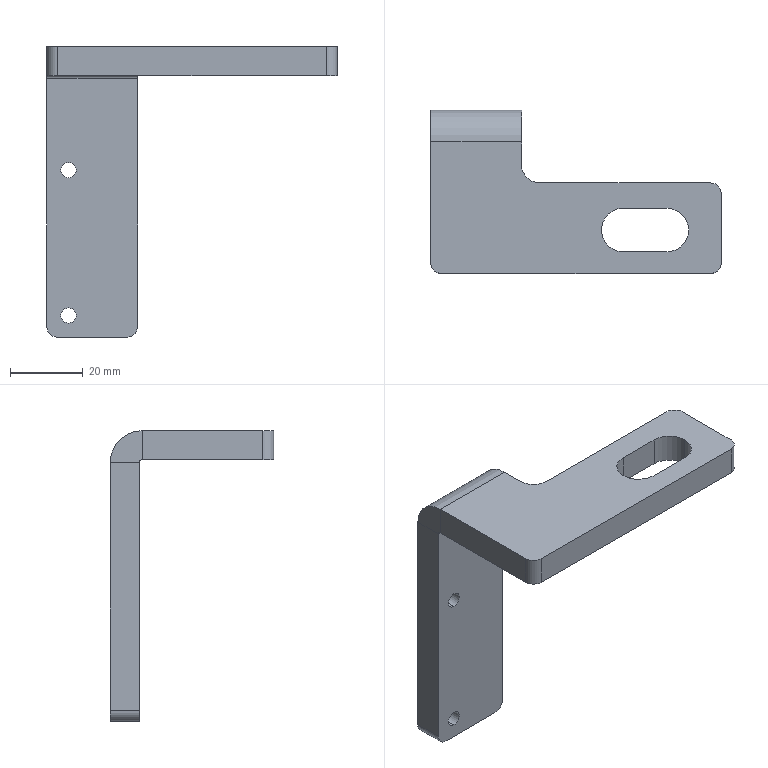Part | 1 solid | 31 faces | box 80 x 45 x 80 mm | volume 31681 mm3 | plane 16 | cylinder 15 | commonest cylinder face diameters 6 x5 4.2 x4 12 x3 1.473 x1 10 x1 17.473 x1
STEP:
#1=CARTESIAN_POINT('',(25.,-4.5,-8.));
#2=VERTEX_POINT('',#1);
#3=CARTESIAN_POINT('',(31.,-10.5,-8.));
#4=VERTEX_POINT('',#3);
#5=CARTESIAN_POINT('',(25.,-10.5,-8.));
#6=DIRECTION('',(0.,0.,-1.));
#7=DIRECTION('',(-1.,0.,0.));
#8=AXIS2_PLACEMENT_3D('',#5,#6,#7);
#9=CIRCLE('',#8,6.);
#10=EDGE_CURVE('',#2,#4,#9,.T.);
#11=ORIENTED_EDGE('',*,*,#10,.T.);
#12=CARTESIAN_POINT('',(31.,-10.5,0.));
#13=VERTEX_POINT('',#12);
#14=CARTESIAN_POINT('',(31.,-10.5,-30.));
#15=DIRECTION('',(0.,0.,1.));
#16=VECTOR('',#15,1000.);
#17=LINE('',#14,#16);
#18=EDGE_CURVE('',#4,#13,#17,.T.);
#19=ORIENTED_EDGE('',*,*,#18,.T.);
#20=CARTESIAN_POINT('',(25.,-4.5,0.));
#21=VERTEX_POINT('',#20);
#22=CARTESIAN_POINT('',(25.,-10.5,0.));
#23=DIRECTION('',(0.,0.,1.));
#24=DIRECTION('',(1.,0.,0.));
#25=AXIS2_PLACEMENT_3D('',#22,#23,#24);
#26=CIRCLE('',#25,6.);
#27=EDGE_CURVE('',#13,#21,#26,.T.);
#28=ORIENTED_EDGE('',*,*,#27,.T.);
#29=CARTESIAN_POINT('',(25.,-4.5,-30.));
#30=DIRECTION('',(0.,0.,1.));
#31=VECTOR('',#30,1000.);
#32=LINE('',#29,#31);
#33=EDGE_CURVE('',#2,#21,#32,.T.);
#34=ORIENTED_EDGE('',*,*,#33,.F.);
#35=EDGE_LOOP('',(#11,#19,#28,#34));
#36=FACE_OUTER_BOUND('',#35,.T.);
#37=CARTESIAN_POINT('',(25.,-10.5,-30.));
#38=DIRECTION('',(0.,0.,1.));
#39=DIRECTION('',(1.,0.,0.));
#40=AXIS2_PLACEMENT_3D('',#37,#38,#39);
#41=CYLINDRICAL_SURFACE('',#40,6.);
#42=ADVANCED_FACE('',(#36),#41,.F.);
#43=CARTESIAN_POINT('',(-34.,14.5,-76.1));
#44=VERTEX_POINT('',#43);
#45=CARTESIAN_POINT('',(-34.,14.5,-71.9));
#46=VERTEX_POINT('',#45);
#47=CARTESIAN_POINT('',(-34.,14.5,-74.));
#48=DIRECTION('',(0.,1.,0.));
#49=DIRECTION('',(0.,0.,1.));
#50=AXIS2_PLACEMENT_3D('',#47,#48,#49);
#51=CIRCLE('',#50,2.1);
#52=EDGE_CURVE('',#44,#46,#51,.T.);
#53=ORIENTED_EDGE('',*,*,#52,.F.);
#54=CARTESIAN_POINT('',(-34.,22.5,-76.1));
#55=VERTEX_POINT('',#54);
#56=CARTESIAN_POINT('',(-34.,22.5,-76.1));
#57=DIRECTION('',(0.,1.,0.));
#58=VECTOR('',#57,1000.);
#59=LINE('',#56,#58);
#60=EDGE_CURVE('',#44,#55,#59,.T.);
#61=ORIENTED_EDGE('',*,*,#60,.T.);
#62=CARTESIAN_POINT('',(-34.,22.5,-71.9));
#63=VERTEX_POINT('',#62);
#64=CARTESIAN_POINT('',(-34.,22.5,-74.));
#65=DIRECTION('',(0.,1.,0.));
#66=DIRECTION('',(0.,0.,1.));
#67=AXIS2_PLACEMENT_3D('',#64,#65,#66);
#68=CIRCLE('',#67,2.1);
#69=EDGE_CURVE('',#55,#63,#68,.T.);
#70=ORIENTED_EDGE('',*,*,#69,.T.);
#71=CARTESIAN_POINT('',(-34.,22.5,-71.9));
#72=DIRECTION('',(0.,1.,0.));
#73=VECTOR('',#72,1000.);
#74=LINE('',#71,#73);
#75=EDGE_CURVE('',#46,#63,#74,.T.);
#76=ORIENTED_EDGE('',*,*,#75,.F.);
#77=EDGE_LOOP('',(#53,#61,#70,#76));
#78=FACE_OUTER_BOUND('',#77,.T.);
#79=CARTESIAN_POINT('',(-34.,22.5,-74.));
#80=DIRECTION('',(0.,1.,0.));
#81=DIRECTION('',(0.,0.,1.));
#82=AXIS2_PLACEMENT_3D('',#79,#80,#81);
#83=CYLINDRICAL_SURFACE('',#82,2.1);
#84=ADVANCED_FACE('',(#78),#83,.F.);
#85=CARTESIAN_POINT('',(-34.,14.5,-36.1));
#86=VERTEX_POINT('',#85);
#87=CARTESIAN_POINT('',(-34.,14.5,-31.9));
#88=VERTEX_POINT('',#87);
#89=CARTESIAN_POINT('',(-34.,14.5,-34.));
#90=DIRECTION('',(0.,1.,0.));
#91=DIRECTION('',(0.,0.,1.));
#92=AXIS2_PLACEMENT_3D('',#89,#90,#91);
#93=CIRCLE('',#92,2.1);
#94=EDGE_CURVE('',#86,#88,#93,.T.);
#95=ORIENTED_EDGE('',*,*,#94,.F.);
#96=CARTESIAN_POINT('',(-34.,22.5,-36.1));
#97=VERTEX_POINT('',#96);
#98=CARTESIAN_POINT('',(-34.,22.5,-36.1));
#99=DIRECTION('',(0.,1.,0.));
#100=VECTOR('',#99,1000.);
#101=LINE('',#98,#100);
#102=EDGE_CURVE('',#86,#97,#101,.T.);
#103=ORIENTED_EDGE('',*,*,#102,.T.);
#104=CARTESIAN_POINT('',(-34.,22.5,-31.9));
#105=VERTEX_POINT('',#104);
#106=CARTESIAN_POINT('',(-34.,22.5,-34.));
#107=DIRECTION('',(0.,1.,0.));
#108=DIRECTION('',(0.,0.,1.));
#109=AXIS2_PLACEMENT_3D('',#106,#107,#108);
#110=CIRCLE('',#109,2.1);
#111=EDGE_CURVE('',#97,#105,#110,.T.);
#112=ORIENTED_EDGE('',*,*,#111,.T.);
#113=CARTESIAN_POINT('',(-34.,22.5,-31.9));
#114=DIRECTION('',(0.,1.,0.));
#115=VECTOR('',#114,1000.);
#116=LINE('',#113,#115);
#117=EDGE_CURVE('',#88,#105,#116,.T.);
#118=ORIENTED_EDGE('',*,*,#117,.F.);
#119=EDGE_LOOP('',(#95,#103,#112,#118));
#120=FACE_OUTER_BOUND('',#119,.T.);
#121=CARTESIAN_POINT('',(-34.,22.5,-34.));
#122=DIRECTION('',(0.,1.,0.));
#123=DIRECTION('',(0.,0.,1.));
#124=AXIS2_PLACEMENT_3D('',#121,#122,#123);
#125=CYLINDRICAL_SURFACE('',#124,2.1);
#126=ADVANCED_FACE('',(#120),#125,.F.);
#127=CARTESIAN_POINT('',(-15.,7.5,0.));
#128=VERTEX_POINT('',#127);
#129=CARTESIAN_POINT('',(-15.,13.763,0.));
#130=VERTEX_POINT('',#129);
#131=CARTESIAN_POINT('',(-15.,2.5,0.));
#132=DIRECTION('',(0.,1.,0.));
#133=VECTOR('',#132,1000.);
#134=LINE('',#131,#133);
#135=EDGE_CURVE('',#128,#130,#134,.T.);
#136=ORIENTED_EDGE('',*,*,#135,.F.);
#137=CARTESIAN_POINT('',(-15.,7.5,-8.));
#138=VERTEX_POINT('',#137);
#139=CARTESIAN_POINT('',(-15.,7.5,-8.));
#140=DIRECTION('',(0.,0.,-1.));
#141=VECTOR('',#140,1000.);
#142=LINE('',#139,#141);
#143=EDGE_CURVE('',#128,#138,#142,.T.);
#144=ORIENTED_EDGE('',*,*,#143,.T.);
#145=CARTESIAN_POINT('',(-15.,13.763,-8.));
#146=VERTEX_POINT('',#145);
#147=CARTESIAN_POINT('',(-15.,0.,-8.));
#148=DIRECTION('',(0.,1.,0.));
#149=VECTOR('',#148,1000.);
#150=LINE('',#147,#149);
#151=EDGE_CURVE('',#138,#146,#150,.T.);
#152=ORIENTED_EDGE('',*,*,#151,.T.);
#153=CARTESIAN_POINT('',(-15.,13.763,-8.));
#154=DIRECTION('',(0.,0.,1.));
#155=VECTOR('',#154,1000.);
#156=LINE('',#153,#155);
#157=EDGE_CURVE('',#146,#130,#156,.T.);
#158=ORIENTED_EDGE('',*,*,#157,.T.);
#159=EDGE_LOOP('',(#136,#144,#152,#158));
#160=FACE_OUTER_BOUND('',#159,.T.);
#161=CARTESIAN_POINT('',(-15.,2.5,0.));
#162=DIRECTION('',(-1.,0.,0.));
#163=DIRECTION('',(0.,0.,1.));
#164=AXIS2_PLACEMENT_3D('',#161,#162,#163);
#165=PLANE('',#164);
#166=ADVANCED_FACE('',(#160),#165,.F.);
#167=CARTESIAN_POINT('',(-15.,14.5,-77.));
#168=VERTEX_POINT('',#167);
#169=CARTESIAN_POINT('',(-15.,14.5,-8.737));
#170=VERTEX_POINT('',#169);
#171=CARTESIAN_POINT('',(-15.,14.5,0.));
#172=DIRECTION('',(0.,0.,1.));
#173=VECTOR('',#172,1000.);
#174=LINE('',#171,#173);
#175=EDGE_CURVE('',#168,#170,#174,.T.);
#176=ORIENTED_EDGE('',*,*,#175,.F.);
#177=CARTESIAN_POINT('',(-15.,22.5,-77.));
#178=VERTEX_POINT('',#177);
#179=CARTESIAN_POINT('',(-15.,22.5,-77.));
#180=DIRECTION('',(0.,1.,0.));
#181=VECTOR('',#180,1000.);
#182=LINE('',#179,#181);
#183=EDGE_CURVE('',#168,#178,#182,.T.);
#184=ORIENTED_EDGE('',*,*,#183,.T.);
#185=CARTESIAN_POINT('',(-15.,22.5,-8.737));
#186=VERTEX_POINT('',#185);
#187=CARTESIAN_POINT('',(-15.,22.5,0.));
#188=DIRECTION('',(0.,0.,1.));
#189=VECTOR('',#188,1000.);
#190=LINE('',#187,#189);
#191=EDGE_CURVE('',#178,#186,#190,.T.);
#192=ORIENTED_EDGE('',*,*,#191,.T.);
#193=CARTESIAN_POINT('',(-15.,22.5,-8.737));
#194=DIRECTION('',(0.,-1.,0.));
#195=VECTOR('',#194,1000.);
#196=LINE('',#193,#195);
#197=EDGE_CURVE('',#186,#170,#196,.T.);
#198=ORIENTED_EDGE('',*,*,#197,.T.);
#199=EDGE_LOOP('',(#176,#184,#192,#198));
#200=FACE_OUTER_BOUND('',#199,.T.);
#201=CARTESIAN_POINT('',(-15.,2.5,0.));
#202=DIRECTION('',(-1.,0.,0.));
#203=DIRECTION('',(0.,0.,1.));
#204=AXIS2_PLACEMENT_3D('',#201,#202,#203);
#205=PLANE('',#204);
#206=ADVANCED_FACE('',(#200),#205,.F.);
#207=CARTESIAN_POINT('',(40.,-19.5,0.));
#208=VERTEX_POINT('',#207);
#209=CARTESIAN_POINT('',(40.,-0.5,0.));
#210=VERTEX_POINT('',#209);
#211=CARTESIAN_POINT('',(40.,-22.5,0.));
#212=DIRECTION('',(0.,1.,0.));
#213=VECTOR('',#212,1000.);
#214=LINE('',#211,#213);
#215=EDGE_CURVE('',#208,#210,#214,.T.);
#216=ORIENTED_EDGE('',*,*,#215,.F.);
#217=CARTESIAN_POINT('',(40.,-19.5,-8.));
#218=VERTEX_POINT('',#217);
#219=CARTESIAN_POINT('',(40.,-19.5,-8.));
#220=DIRECTION('',(0.,0.,-1.));
#221=VECTOR('',#220,1000.);
#222=LINE('',#219,#221);
#223=EDGE_CURVE('',#208,#218,#222,.T.);
#224=ORIENTED_EDGE('',*,*,#223,.T.);
#225=CARTESIAN_POINT('',(40.,-0.5,-8.));
#226=VERTEX_POINT('',#225);
#227=CARTESIAN_POINT('',(40.,-22.5,-8.));
#228=DIRECTION('',(0.,1.,0.));
#229=VECTOR('',#228,1000.);
#230=LINE('',#227,#229);
#231=EDGE_CURVE('',#218,#226,#230,.T.);
#232=ORIENTED_EDGE('',*,*,#231,.T.);
#233=CARTESIAN_POINT('',(40.,-0.5,0.));
#234=DIRECTION('',(0.,0.,1.));
#235=VECTOR('',#234,1000.);
#236=LINE('',#233,#235);
#237=EDGE_CURVE('',#226,#210,#236,.T.);
#238=ORIENTED_EDGE('',*,*,#237,.T.);
#239=EDGE_LOOP('',(#216,#224,#232,#238));
#240=FACE_OUTER_BOUND('',#239,.T.);
#241=CARTESIAN_POINT('',(40.,-22.5,-8.));
#242=DIRECTION('',(1.,0.,0.));
#243=DIRECTION('',(0.,0.,-1.));
#244=AXIS2_PLACEMENT_3D('',#241,#242,#243);
#245=PLANE('',#244);
#246=ADVANCED_FACE('',(#240),#245,.T.);
#247=ORIENTED_EDGE('',*,*,#10,.F.);
#248=CARTESIAN_POINT('',(13.,-4.5,-8.));
#249=VERTEX_POINT('',#248);
#250=CARTESIAN_POINT('',(0.,-4.5,-8.));
#251=DIRECTION('',(1.,0.,0.));
#252=VECTOR('',#251,1000.);
#253=LINE('',#250,#252);
#254=EDGE_CURVE('',#249,#2,#253,.T.);
#255=ORIENTED_EDGE('',*,*,#254,.F.);
#256=CARTESIAN_POINT('',(13.,-16.5,-8.));
#257=VERTEX_POINT('',#256);
#258=CARTESIAN_POINT('',(13.,-10.5,-8.));
#259=DIRECTION('',(0.,0.,-1.));
#260=DIRECTION('',(-1.,0.,0.));
#261=AXIS2_PLACEMENT_3D('',#258,#259,#260);
#262=CIRCLE('',#261,6.);
#263=EDGE_CURVE('',#257,#249,#262,.T.);
#264=ORIENTED_EDGE('',*,*,#263,.F.);
#265=CARTESIAN_POINT('',(25.,-16.5,-8.));
#266=VERTEX_POINT('',#265);
#267=CARTESIAN_POINT('',(0.,-16.5,-8.));
#268=DIRECTION('',(-1.,0.,0.));
#269=VECTOR('',#268,1000.);
#270=LINE('',#267,#269);
#271=EDGE_CURVE('',#266,#257,#270,.T.);
#272=ORIENTED_EDGE('',*,*,#271,.F.);
#273=CARTESIAN_POINT('',(25.,-10.5,-8.));
#274=DIRECTION('',(0.,0.,-1.));
#275=DIRECTION('',(-1.,0.,0.));
#276=AXIS2_PLACEMENT_3D('',#273,#274,#275);
#277=CIRCLE('',#276,6.);
#278=EDGE_CURVE('',#4,#266,#277,.T.);
#279=ORIENTED_EDGE('',*,*,#278,.F.);
#280=EDGE_LOOP('',(#247,#255,#264,#272,#279));
#281=FACE_BOUND('',#280,.T.);
#282=CARTESIAN_POINT('',(-37.,-22.5,-8.));
#283=VERTEX_POINT('',#282);
#284=CARTESIAN_POINT('',(37.,-22.5,-8.));
#285=VERTEX_POINT('',#284);
#286=CARTESIAN_POINT('',(-40.,-22.5,-8.));
#287=DIRECTION('',(1.,0.,0.));
#288=VECTOR('',#287,1000.);
#289=LINE('',#286,#288);
#290=EDGE_CURVE('',#283,#285,#289,.T.);
#291=ORIENTED_EDGE('',*,*,#290,.F.);
#292=CARTESIAN_POINT('',(-40.,-19.5,-8.));
#293=VERTEX_POINT('',#292);
#294=CARTESIAN_POINT('',(-37.,-19.5,-8.));
#295=DIRECTION('',(0.,0.,-1.));
#296=DIRECTION('',(-1.,0.,0.));
#297=AXIS2_PLACEMENT_3D('',#294,#295,#296);
#298=CIRCLE('',#297,3.);
#299=EDGE_CURVE('',#283,#293,#298,.T.);
#300=ORIENTED_EDGE('',*,*,#299,.T.);
#301=CARTESIAN_POINT('',(-40.,13.763,-8.));
#302=VERTEX_POINT('',#301);
#303=CARTESIAN_POINT('',(-40.,-22.5,-8.));
#304=DIRECTION('',(0.,-1.,0.));
#305=VECTOR('',#304,1000.);
#306=LINE('',#303,#305);
#307=EDGE_CURVE('',#302,#293,#306,.T.);
#308=ORIENTED_EDGE('',*,*,#307,.F.);
#309=CARTESIAN_POINT('',(40.,13.763,-8.));
#310=DIRECTION('',(-1.,0.,0.));
#311=VECTOR('',#310,1000.);
#312=LINE('',#309,#311);
#313=EDGE_CURVE('',#146,#302,#312,.T.);
#314=ORIENTED_EDGE('',*,*,#313,.F.);
#315=ORIENTED_EDGE('',*,*,#151,.F.);
#316=CARTESIAN_POINT('',(-10.,2.5,-8.));
#317=VERTEX_POINT('',#316);
#318=CARTESIAN_POINT('',(-10.,7.5,-8.));
#319=DIRECTION('',(0.,0.,1.));
#320=DIRECTION('',(-1.,0.,0.));
#321=AXIS2_PLACEMENT_3D('',#318,#319,#320);
#322=CIRCLE('',#321,5.);
#323=EDGE_CURVE('',#138,#317,#322,.T.);
#324=ORIENTED_EDGE('',*,*,#323,.T.);
#325=CARTESIAN_POINT('',(37.,2.5,-8.));
#326=VERTEX_POINT('',#325);
#327=CARTESIAN_POINT('',(0.,2.5,-8.));
#328=DIRECTION('',(-1.,0.,0.));
#329=VECTOR('',#328,1000.);
#330=LINE('',#327,#329);
#331=EDGE_CURVE('',#326,#317,#330,.T.);
#332=ORIENTED_EDGE('',*,*,#331,.F.);
#333=CARTESIAN_POINT('',(37.,-0.5,-8.));
#334=DIRECTION('',(0.,0.,-1.));
#335=DIRECTION('',(-1.,0.,0.));
#336=AXIS2_PLACEMENT_3D('',#333,#334,#335);
#337=CIRCLE('',#336,3.);
#338=EDGE_CURVE('',#326,#226,#337,.T.);
#339=ORIENTED_EDGE('',*,*,#338,.T.);
#340=ORIENTED_EDGE('',*,*,#231,.F.);
#341=CARTESIAN_POINT('',(37.,-19.5,-8.));
#342=DIRECTION('',(0.,0.,-1.));
#343=DIRECTION('',(-1.,0.,0.));
#344=AXIS2_PLACEMENT_3D('',#341,#342,#343);
#345=CIRCLE('',#344,3.);
#346=EDGE_CURVE('',#218,#285,#345,.T.);
#347=ORIENTED_EDGE('',*,*,#346,.T.);
#348=EDGE_LOOP('',(#291,#300,#308,#314,#315,#324,#332,#339,#340,#347));
#349=FACE_OUTER_BOUND('',#348,.T.);
#350=CARTESIAN_POINT('',(0.,0.,-8.));
#351=DIRECTION('',(0.,0.,-1.));
#352=DIRECTION('',(-1.,0.,0.));
#353=AXIS2_PLACEMENT_3D('',#350,#351,#352);
#354=PLANE('',#353);
#355=ADVANCED_FACE('',(#281,#349),#354,.T.);
#356=CARTESIAN_POINT('',(13.,-4.5,0.));
#357=VERTEX_POINT('',#356);
#358=CARTESIAN_POINT('',(25.,-4.5,0.));
#359=DIRECTION('',(-1.,0.,0.));
#360=VECTOR('',#359,1000.);
#361=LINE('',#358,#360);
#362=EDGE_CURVE('',#21,#357,#361,.T.);
#363=ORIENTED_EDGE('',*,*,#362,.F.);
#364=ORIENTED_EDGE('',*,*,#27,.F.);
#365=CARTESIAN_POINT('',(25.,-16.5,0.));
#366=VERTEX_POINT('',#365);
#367=CARTESIAN_POINT('',(25.,-10.5,0.));
#368=DIRECTION('',(0.,0.,1.));
#369=DIRECTION('',(1.,0.,0.));
#370=AXIS2_PLACEMENT_3D('',#367,#368,#369);
#371=CIRCLE('',#370,6.);
#372=EDGE_CURVE('',#366,#13,#371,.T.);
#373=ORIENTED_EDGE('',*,*,#372,.F.);
#374=CARTESIAN_POINT('',(13.,-16.5,0.));
#375=VERTEX_POINT('',#374);
#376=CARTESIAN_POINT('',(25.,-16.5,0.));
#377=DIRECTION('',(1.,0.,0.));
#378=VECTOR('',#377,1000.);
#379=LINE('',#376,#378);
#380=EDGE_CURVE('',#375,#366,#379,.T.);
#381=ORIENTED_EDGE('',*,*,#380,.F.);
#382=CARTESIAN_POINT('',(13.,-10.5,0.));
#383=DIRECTION('',(0.,0.,1.));
#384=DIRECTION('',(1.,0.,0.));
#385=AXIS2_PLACEMENT_3D('',#382,#383,#384);
#386=CIRCLE('',#385,6.);
#387=EDGE_CURVE('',#357,#375,#386,.T.);
#388=ORIENTED_EDGE('',*,*,#387,.F.);
#389=EDGE_LOOP('',(#363,#364,#373,#381,#388));
#390=FACE_BOUND('',#389,.T.);
#391=CARTESIAN_POINT('',(-40.,13.763,0.));
#392=VERTEX_POINT('',#391);
#393=CARTESIAN_POINT('',(-40.,-19.5,0.));
#394=VERTEX_POINT('',#393);
#395=CARTESIAN_POINT('',(-40.,-22.5,0.));
#396=DIRECTION('',(0.,-1.,0.));
#397=VECTOR('',#396,1000.);
#398=LINE('',#395,#397);
#399=EDGE_CURVE('',#392,#394,#398,.T.);
#400=ORIENTED_EDGE('',*,*,#399,.T.);
#401=CARTESIAN_POINT('',(-37.,-22.5,0.));
#402=VERTEX_POINT('',#401);
#403=CARTESIAN_POINT('',(-37.,-19.5,0.));
#404=DIRECTION('',(0.,0.,1.));
#405=DIRECTION('',(-1.,0.,0.));
#406=AXIS2_PLACEMENT_3D('',#403,#404,#405);
#407=CIRCLE('',#406,3.);
#408=EDGE_CURVE('',#394,#402,#407,.T.);
#409=ORIENTED_EDGE('',*,*,#408,.T.);
#410=CARTESIAN_POINT('',(37.,-22.5,0.));
#411=VERTEX_POINT('',#410);
#412=CARTESIAN_POINT('',(-40.,-22.5,0.));
#413=DIRECTION('',(1.,0.,0.));
#414=VECTOR('',#413,1000.);
#415=LINE('',#412,#414);
#416=EDGE_CURVE('',#402,#411,#415,.T.);
#417=ORIENTED_EDGE('',*,*,#416,.T.);
#418=CARTESIAN_POINT('',(37.,-19.5,0.));
#419=DIRECTION('',(0.,0.,1.));
#420=DIRECTION('',(-1.,0.,0.));
#421=AXIS2_PLACEMENT_3D('',#418,#419,#420);
#422=CIRCLE('',#421,3.);
#423=EDGE_CURVE('',#411,#208,#422,.T.);
#424=ORIENTED_EDGE('',*,*,#423,.T.);
#425=ORIENTED_EDGE('',*,*,#215,.T.);
#426=CARTESIAN_POINT('',(37.,2.5,0.));
#427=VERTEX_POINT('',#426);
#428=CARTESIAN_POINT('',(37.,-0.5,0.));
#429=DIRECTION('',(0.,0.,1.));
#430=DIRECTION('',(-1.,0.,0.));
#431=AXIS2_PLACEMENT_3D('',#428,#429,#430);
#432=CIRCLE('',#431,3.);
#433=EDGE_CURVE('',#210,#427,#432,.T.);
#434=ORIENTED_EDGE('',*,*,#433,.T.);
#435=CARTESIAN_POINT('',(-10.,2.5,0.));
#436=VERTEX_POINT('',#435);
#437=CARTESIAN_POINT('',(-15.,2.5,0.));
#438=DIRECTION('',(1.,0.,0.));
#439=VECTOR('',#438,1000.);
#440=LINE('',#437,#439);
#441=EDGE_CURVE('',#436,#427,#440,.T.);
#442=ORIENTED_EDGE('',*,*,#441,.F.);
#443=CARTESIAN_POINT('',(-10.,7.5,0.));
#444=DIRECTION('',(0.,0.,-1.));
#445=DIRECTION('',(-1.,0.,0.));
#446=AXIS2_PLACEMENT_3D('',#443,#444,#445);
#447=CIRCLE('',#446,5.);
#448=EDGE_CURVE('',#436,#128,#447,.T.);
#449=ORIENTED_EDGE('',*,*,#448,.T.);
#450=ORIENTED_EDGE('',*,*,#135,.T.);
#451=CARTESIAN_POINT('',(40.,13.763,0.));
#452=DIRECTION('',(-1.,0.,0.));
#453=VECTOR('',#452,1000.);
#454=LINE('',#451,#453);
#455=EDGE_CURVE('',#130,#392,#454,.T.);
#456=ORIENTED_EDGE('',*,*,#455,.T.);
#457=EDGE_LOOP('',(#400,#409,#417,#424,#425,#434,#442,#449,#450,#456));
#458=FACE_OUTER_BOUND('',#457,.T.);
#459=CARTESIAN_POINT('',(0.,0.,0.));
#460=DIRECTION('',(0.,0.,-1.));
#461=DIRECTION('',(-1.,0.,0.));
#462=AXIS2_PLACEMENT_3D('',#459,#460,#461);
#463=PLANE('',#462);
#464=ADVANCED_FACE('',(#390,#458),#463,.F.);
#465=ORIENTED_EDGE('',*,*,#416,.F.);
#466=CARTESIAN_POINT('',(-37.,-22.5,-8.));
#467=DIRECTION('',(0.,0.,-1.));
#468=VECTOR('',#467,1000.);
#469=LINE('',#466,#468);
#470=EDGE_CURVE('',#402,#283,#469,.T.);
#471=ORIENTED_EDGE('',*,*,#470,.T.);
#472=ORIENTED_EDGE('',*,*,#290,.T.);
#473=CARTESIAN_POINT('',(37.,-22.5,-8.));
#474=DIRECTION('',(0.,0.,1.));
#475=VECTOR('',#474,1000.);
#476=LINE('',#473,#475);
#477=EDGE_CURVE('',#285,#411,#476,.T.);
#478=ORIENTED_EDGE('',*,*,#477,.T.);
#479=EDGE_LOOP('',(#465,#471,#472,#478));
#480=FACE_OUTER_BOUND('',#479,.T.);
#481=CARTESIAN_POINT('',(-40.,-22.5,-8.));
#482=DIRECTION('',(0.,-1.,0.));
#483=DIRECTION('',(0.,0.,-1.));
#484=AXIS2_PLACEMENT_3D('',#481,#482,#483);
#485=PLANE('',#484);
#486=ADVANCED_FACE('',(#480),#485,.T.);
#487=ORIENTED_EDGE('',*,*,#307,.T.);
#488=CARTESIAN_POINT('',(-40.,-19.5,-8.));
#489=DIRECTION('',(0.,0.,1.));
#490=VECTOR('',#489,1000.);
#491=LINE('',#488,#490);
#492=EDGE_CURVE('',#293,#394,#491,.T.);
#493=ORIENTED_EDGE('',*,*,#492,.T.);
#494=ORIENTED_EDGE('',*,*,#399,.F.);
#495=CARTESIAN_POINT('',(-40.,13.763,-8.));
#496=DIRECTION('',(0.,0.,1.));
#497=VECTOR('',#496,1000.);
#498=LINE('',#495,#497);
#499=EDGE_CURVE('',#302,#392,#498,.T.);
#500=ORIENTED_EDGE('',*,*,#499,.F.);
#501=EDGE_LOOP('',(#487,#493,#494,#500));
#502=FACE_OUTER_BOUND('',#501,.T.);
#503=CARTESIAN_POINT('',(-40.,-22.5,-8.));
#504=DIRECTION('',(-1.,0.,0.));
#505=DIRECTION('',(0.,0.,1.));
#506=AXIS2_PLACEMENT_3D('',#503,#504,#505);
#507=PLANE('',#506);
#508=ADVANCED_FACE('',(#502),#507,.T.);
#509=CARTESIAN_POINT('',(-40.,14.5,-8.737));
#510=VERTEX_POINT('',#509);
#511=CARTESIAN_POINT('',(-40.,22.5,-8.737));
#512=VERTEX_POINT('',#511);
#513=CARTESIAN_POINT('',(-40.,22.5,-8.737));
#514=DIRECTION('',(0.,1.,0.));
#515=VECTOR('',#514,1000.);
#516=LINE('',#513,#515);
#517=EDGE_CURVE('',#510,#512,#516,.T.);
#518=ORIENTED_EDGE('',*,*,#517,.F.);
#519=CARTESIAN_POINT('',(-40.,13.763,-8.737));
#520=DIRECTION('',(-1.,0.,0.));
#521=DIRECTION('',(0.,0.,-1.));
#522=AXIS2_PLACEMENT_3D('',#519,#520,#521);
#523=CIRCLE('',#522,0.7366);
#524=EDGE_CURVE('',#302,#510,#523,.T.);
#525=ORIENTED_EDGE('',*,*,#524,.F.);
#526=ORIENTED_EDGE('',*,*,#499,.T.);
#527=CARTESIAN_POINT('',(-40.,13.763,-8.737));
#528=DIRECTION('',(-1.,0.,0.));
#529=DIRECTION('',(0.,0.,-1.));
#530=AXIS2_PLACEMENT_3D('',#527,#528,#529);
#531=CIRCLE('',#530,8.737);
#532=EDGE_CURVE('',#392,#512,#531,.T.);
#533=ORIENTED_EDGE('',*,*,#532,.T.);
#534=EDGE_LOOP('',(#518,#525,#526,#533));
#535=FACE_OUTER_BOUND('',#534,.T.);
#536=CARTESIAN_POINT('',(-40.,13.763,-8.737));
#537=DIRECTION('',(-1.,0.,0.));
#538=DIRECTION('',(0.,0.,1.));
#539=AXIS2_PLACEMENT_3D('',#536,#537,#538);
#540=PLANE('',#539);
#541=ADVANCED_FACE('',(#535),#540,.T.);
#542=CARTESIAN_POINT('',(-15.,13.763,-8.737));
#543=DIRECTION('',(1.,0.,0.));
#544=DIRECTION('',(0.,0.,1.));
#545=AXIS2_PLACEMENT_3D('',#542,#543,#544);
#546=CIRCLE('',#545,8.737);
#547=EDGE_CURVE('',#186,#130,#546,.T.);
#548=ORIENTED_EDGE('',*,*,#547,.F.);
#549=CARTESIAN_POINT('',(0.,22.5,-8.737));
#550=DIRECTION('',(1.,0.,0.));
#551=VECTOR('',#550,1000.);
#552=LINE('',#549,#551);
#553=EDGE_CURVE('',#512,#186,#552,.T.);
#554=ORIENTED_EDGE('',*,*,#553,.F.);
#555=ORIENTED_EDGE('',*,*,#532,.F.);
#556=ORIENTED_EDGE('',*,*,#455,.F.);
#557=EDGE_LOOP('',(#548,#554,#555,#556));
#558=FACE_OUTER_BOUND('',#557,.T.);
#559=CARTESIAN_POINT('',(40.,13.763,-8.737));
#560=DIRECTION('',(1.,0.,0.));
#561=DIRECTION('',(0.,1.,0.));
#562=AXIS2_PLACEMENT_3D('',#559,#560,#561);
#563=CYLINDRICAL_SURFACE('',#562,8.737);
#564=ADVANCED_FACE('',(#558),#563,.T.);
#565=CARTESIAN_POINT('',(-40.,14.5,-8.737));
#566=DIRECTION('',(1.,0.,0.));
#567=VECTOR('',#566,1000.);
#568=LINE('',#565,#567);
#569=EDGE_CURVE('',#510,#170,#568,.T.);
#570=ORIENTED_EDGE('',*,*,#569,.T.);
#571=CARTESIAN_POINT('',(-15.,13.763,-8.737));
#572=DIRECTION('',(1.,0.,0.));
#573=DIRECTION('',(0.,0.,1.));
#574=AXIS2_PLACEMENT_3D('',#571,#572,#573);
#575=CIRCLE('',#574,0.7366);
#576=EDGE_CURVE('',#170,#146,#575,.T.);
#577=ORIENTED_EDGE('',*,*,#576,.T.);
#578=ORIENTED_EDGE('',*,*,#313,.T.);
#579=ORIENTED_EDGE('',*,*,#524,.T.);
#580=EDGE_LOOP('',(#570,#577,#578,#579));
#581=FACE_OUTER_BOUND('',#580,.T.);
#582=CARTESIAN_POINT('',(40.,13.763,-8.737));
#583=DIRECTION('',(1.,0.,0.));
#584=DIRECTION('',(0.,1.,0.));
#585=AXIS2_PLACEMENT_3D('',#582,#583,#584);
#586=CYLINDRICAL_SURFACE('',#585,0.7366);
#587=ADVANCED_FACE('',(#581),#586,.F.);
#588=CARTESIAN_POINT('',(-40.,22.5,-77.));
#589=VERTEX_POINT('',#588);
#590=CARTESIAN_POINT('',(-40.,22.5,-80.));
#591=DIRECTION('',(0.,0.,-1.));
#592=VECTOR('',#591,1000.);
#593=LINE('',#590,#592);
#594=EDGE_CURVE('',#512,#589,#593,.T.);
#595=ORIENTED_EDGE('',*,*,#594,.T.);
#596=CARTESIAN_POINT('',(-40.,14.5,-77.));
#597=VERTEX_POINT('',#596);
#598=CARTESIAN_POINT('',(-40.,22.5,-77.));
#599=DIRECTION('',(0.,-1.,0.));
#600=VECTOR('',#599,1000.);
#601=LINE('',#598,#600);
#602=EDGE_CURVE('',#589,#597,#601,.T.);
#603=ORIENTED_EDGE('',*,*,#602,.T.);
#604=CARTESIAN_POINT('',(-40.,14.5,0.));
#605=DIRECTION('',(0.,0.,-1.));
#606=VECTOR('',#605,1000.);
#607=LINE('',#604,#606);
#608=EDGE_CURVE('',#510,#597,#607,.T.);
#609=ORIENTED_EDGE('',*,*,#608,.F.);
#610=ORIENTED_EDGE('',*,*,#517,.T.);
#611=EDGE_LOOP('',(#595,#603,#609,#610));
#612=FACE_OUTER_BOUND('',#611,.T.);
#613=CARTESIAN_POINT('',(-40.,22.5,-80.));
#614=DIRECTION('',(-1.,0.,0.));
#615=DIRECTION('',(0.,0.,1.));
#616=AXIS2_PLACEMENT_3D('',#613,#614,#615);
#617=PLANE('',#616);
#618=ADVANCED_FACE('',(#612),#617,.T.);
#619=CARTESIAN_POINT('',(-37.,22.5,-80.));
#620=VERTEX_POINT('',#619);
#621=CARTESIAN_POINT('',(-18.,22.5,-80.));
#622=VERTEX_POINT('',#621);
#623=CARTESIAN_POINT('',(40.,22.5,-80.));
#624=DIRECTION('',(1.,0.,0.));
#625=VECTOR('',#624,1000.);
#626=LINE('',#623,#625);
#627=EDGE_CURVE('',#620,#622,#626,.T.);
#628=ORIENTED_EDGE('',*,*,#627,.F.);
#629=CARTESIAN_POINT('',(-37.,22.5,-77.));
#630=DIRECTION('',(0.,1.,0.));
#631=DIRECTION('',(0.,0.,1.));
#632=AXIS2_PLACEMENT_3D('',#629,#630,#631);
#633=CIRCLE('',#632,3.);
#634=EDGE_CURVE('',#620,#589,#633,.T.);
#635=ORIENTED_EDGE('',*,*,#634,.T.);
#636=ORIENTED_EDGE('',*,*,#594,.F.);
#637=ORIENTED_EDGE('',*,*,#553,.T.);
#638=ORIENTED_EDGE('',*,*,#191,.F.);
#639=CARTESIAN_POINT('',(-18.,22.5,-77.));
#640=DIRECTION('',(0.,1.,0.));
#641=DIRECTION('',(0.,0.,1.));
#642=AXIS2_PLACEMENT_3D('',#639,#640,#641);
#643=CIRCLE('',#642,3.);
#644=EDGE_CURVE('',#178,#622,#643,.T.);
#645=ORIENTED_EDGE('',*,*,#644,.T.);
#646=EDGE_LOOP('',(#628,#635,#636,#637,#638,#645));
#647=FACE_OUTER_BOUND('',#646,.T.);
#648=CARTESIAN_POINT('',(-34.,22.5,-74.));
#649=DIRECTION('',(0.,1.,0.));
#650=DIRECTION('',(0.,0.,1.));
#651=AXIS2_PLACEMENT_3D('',#648,#649,#650);
#652=CIRCLE('',#651,2.1);
#653=EDGE_CURVE('',#63,#55,#652,.T.);
#654=ORIENTED_EDGE('',*,*,#653,.F.);
#655=ORIENTED_EDGE('',*,*,#69,.F.);
#656=EDGE_LOOP('',(#654,#655));
#657=FACE_BOUND('',#656,.T.);
#658=CARTESIAN_POINT('',(-34.,22.5,-34.));
#659=DIRECTION('',(0.,1.,0.));
#660=DIRECTION('',(0.,0.,1.));
#661=AXIS2_PLACEMENT_3D('',#658,#659,#660);
#662=CIRCLE('',#661,2.1);
#663=EDGE_CURVE('',#105,#97,#662,.T.);
#664=ORIENTED_EDGE('',*,*,#663,.F.);
#665=ORIENTED_EDGE('',*,*,#111,.F.);
#666=EDGE_LOOP('',(#664,#665));
#667=FACE_BOUND('',#666,.T.);
#668=CARTESIAN_POINT('',(0.,22.5,0.));
#669=DIRECTION('',(0.,1.,0.));
#670=DIRECTION('',(0.,0.,1.));
#671=AXIS2_PLACEMENT_3D('',#668,#669,#670);
#672=PLANE('',#671);
#673=ADVANCED_FACE('',(#647,#657,#667),#672,.T.);
#674=CARTESIAN_POINT('',(-34.,14.5,-74.));
#675=DIRECTION('',(0.,1.,0.));
#676=DIRECTION('',(0.,0.,1.));
#677=AXIS2_PLACEMENT_3D('',#674,#675,#676);
#678=CIRCLE('',#677,2.1);
#679=EDGE_CURVE('',#46,#44,#678,.T.);
#680=ORIENTED_EDGE('',*,*,#679,.T.);
#681=ORIENTED_EDGE('',*,*,#52,.T.);
#682=EDGE_LOOP('',(#680,#681));
#683=FACE_BOUND('',#682,.T.);
#684=CARTESIAN_POINT('',(-34.,14.5,-34.));
#685=DIRECTION('',(0.,1.,0.));
#686=DIRECTION('',(0.,0.,1.));
#687=AXIS2_PLACEMENT_3D('',#684,#685,#686);
#688=CIRCLE('',#687,2.1);
#689=EDGE_CURVE('',#88,#86,#688,.T.);
#690=ORIENTED_EDGE('',*,*,#689,.T.);
#691=ORIENTED_EDGE('',*,*,#94,.T.);
#692=EDGE_LOOP('',(#690,#691));
#693=FACE_BOUND('',#692,.T.);
#694=ORIENTED_EDGE('',*,*,#608,.T.);
#695=CARTESIAN_POINT('',(-37.,14.5,-80.));
#696=VERTEX_POINT('',#695);
#697=CARTESIAN_POINT('',(-37.,14.5,-77.));
#698=DIRECTION('',(0.,-1.,0.));
#699=DIRECTION('',(0.,0.,1.));
#700=AXIS2_PLACEMENT_3D('',#697,#698,#699);
#701=CIRCLE('',#700,3.);
#702=EDGE_CURVE('',#597,#696,#701,.T.);
#703=ORIENTED_EDGE('',*,*,#702,.T.);
#704=CARTESIAN_POINT('',(-18.,14.5,-80.));
#705=VERTEX_POINT('',#704);
#706=CARTESIAN_POINT('',(0.,14.5,-80.));
#707=DIRECTION('',(1.,0.,0.));
#708=VECTOR('',#707,1000.);
#709=LINE('',#706,#708);
#710=EDGE_CURVE('',#696,#705,#709,.T.);
#711=ORIENTED_EDGE('',*,*,#710,.T.);
#712=CARTESIAN_POINT('',(-18.,14.5,-77.));
#713=DIRECTION('',(0.,-1.,0.));
#714=DIRECTION('',(0.,0.,1.));
#715=AXIS2_PLACEMENT_3D('',#712,#713,#714);
#716=CIRCLE('',#715,3.);
#717=EDGE_CURVE('',#705,#168,#716,.T.);
#718=ORIENTED_EDGE('',*,*,#717,.T.);
#719=ORIENTED_EDGE('',*,*,#175,.T.);
#720=ORIENTED_EDGE('',*,*,#569,.F.);
#721=EDGE_LOOP('',(#694,#703,#711,#718,#719,#720));
#722=FACE_OUTER_BOUND('',#721,.T.);
#723=CARTESIAN_POINT('',(0.,14.5,0.));
#724=DIRECTION('',(0.,1.,0.));
#725=DIRECTION('',(0.,0.,1.));
#726=AXIS2_PLACEMENT_3D('',#723,#724,#725);
#727=PLANE('',#726);
#728=ADVANCED_FACE('',(#683,#693,#722),#727,.F.);
#729=ORIENTED_EDGE('',*,*,#710,.F.);
#730=CARTESIAN_POINT('',(-37.,22.5,-80.));
#731=DIRECTION('',(0.,1.,0.));
#732=VECTOR('',#731,1000.);
#733=LINE('',#730,#732);
#734=EDGE_CURVE('',#696,#620,#733,.T.);
#735=ORIENTED_EDGE('',*,*,#734,.T.);
#736=ORIENTED_EDGE('',*,*,#627,.T.);
#737=CARTESIAN_POINT('',(-18.,14.5,-80.));
#738=DIRECTION('',(0.,-1.,0.));
#739=VECTOR('',#738,1000.);
#740=LINE('',#737,#739);
#741=EDGE_CURVE('',#622,#705,#740,.T.);
#742=ORIENTED_EDGE('',*,*,#741,.T.);
#743=EDGE_LOOP('',(#729,#735,#736,#742));
#744=FACE_OUTER_BOUND('',#743,.T.);
#745=CARTESIAN_POINT('',(40.,22.5,-80.));
#746=DIRECTION('',(0.,0.,-1.));
#747=DIRECTION('',(0.,1.,0.));
#748=AXIS2_PLACEMENT_3D('',#745,#746,#747);
#749=PLANE('',#748);
#750=ADVANCED_FACE('',(#744),#749,.T.);
#751=ORIENTED_EDGE('',*,*,#102,.F.);
#752=ORIENTED_EDGE('',*,*,#689,.F.);
#753=ORIENTED_EDGE('',*,*,#117,.T.);
#754=ORIENTED_EDGE('',*,*,#663,.T.);
#755=EDGE_LOOP('',(#751,#752,#753,#754));
#756=FACE_OUTER_BOUND('',#755,.T.);
#757=CARTESIAN_POINT('',(-34.,22.5,-34.));
#758=DIRECTION('',(0.,1.,0.));
#759=DIRECTION('',(0.,0.,1.));
#760=AXIS2_PLACEMENT_3D('',#757,#758,#759);
#761=CYLINDRICAL_SURFACE('',#760,2.1);
#762=ADVANCED_FACE('',(#756),#761,.F.);
#763=ORIENTED_EDGE('',*,*,#60,.F.);
#764=ORIENTED_EDGE('',*,*,#679,.F.);
#765=ORIENTED_EDGE('',*,*,#75,.T.);
#766=ORIENTED_EDGE('',*,*,#653,.T.);
#767=EDGE_LOOP('',(#763,#764,#765,#766));
#768=FACE_OUTER_BOUND('',#767,.T.);
#769=CARTESIAN_POINT('',(-34.,22.5,-74.));
#770=DIRECTION('',(0.,1.,0.));
#771=DIRECTION('',(0.,0.,1.));
#772=AXIS2_PLACEMENT_3D('',#769,#770,#771);
#773=CYLINDRICAL_SURFACE('',#772,2.1);
#774=ADVANCED_FACE('',(#768),#773,.F.);
#775=ORIENTED_EDGE('',*,*,#157,.F.);
#776=ORIENTED_EDGE('',*,*,#576,.F.);
#777=ORIENTED_EDGE('',*,*,#197,.F.);
#778=ORIENTED_EDGE('',*,*,#547,.T.);
#779=EDGE_LOOP('',(#775,#776,#777,#778));
#780=FACE_OUTER_BOUND('',#779,.T.);
#781=CARTESIAN_POINT('',(-15.,2.5,0.));
#782=DIRECTION('',(-1.,0.,0.));
#783=DIRECTION('',(0.,0.,1.));
#784=AXIS2_PLACEMENT_3D('',#781,#782,#783);
#785=PLANE('',#784);
#786=ADVANCED_FACE('',(#780),#785,.F.);
#787=ORIENTED_EDGE('',*,*,#441,.T.);
#788=CARTESIAN_POINT('',(37.,2.5,-8.));
#789=DIRECTION('',(0.,0.,-1.));
#790=VECTOR('',#789,1000.);
#791=LINE('',#788,#790);
#792=EDGE_CURVE('',#427,#326,#791,.T.);
#793=ORIENTED_EDGE('',*,*,#792,.T.);
#794=ORIENTED_EDGE('',*,*,#331,.T.);
#795=CARTESIAN_POINT('',(-10.,2.5,0.));
#796=DIRECTION('',(0.,0.,1.));
#797=VECTOR('',#796,1000.);
#798=LINE('',#795,#797);
#799=EDGE_CURVE('',#317,#436,#798,.T.);
#800=ORIENTED_EDGE('',*,*,#799,.T.);
#801=EDGE_LOOP('',(#787,#793,#794,#800));
#802=FACE_OUTER_BOUND('',#801,.T.);
#803=CARTESIAN_POINT('',(0.,2.5,0.));
#804=DIRECTION('',(0.,-1.,0.));
#805=DIRECTION('',(0.,0.,-1.));
#806=AXIS2_PLACEMENT_3D('',#803,#804,#805);
#807=PLANE('',#806);
#808=ADVANCED_FACE('',(#802),#807,.F.);
#809=ORIENTED_EDGE('',*,*,#18,.F.);
#810=ORIENTED_EDGE('',*,*,#278,.T.);
#811=CARTESIAN_POINT('',(25.,-16.5,-30.));
#812=DIRECTION('',(0.,0.,1.));
#813=VECTOR('',#812,1000.);
#814=LINE('',#811,#813);
#815=EDGE_CURVE('',#266,#366,#814,.T.);
#816=ORIENTED_EDGE('',*,*,#815,.T.);
#817=ORIENTED_EDGE('',*,*,#372,.T.);
#818=EDGE_LOOP('',(#809,#810,#816,#817));
#819=FACE_OUTER_BOUND('',#818,.T.);
#820=CARTESIAN_POINT('',(25.,-10.5,-30.));
#821=DIRECTION('',(0.,0.,1.));
#822=DIRECTION('',(1.,0.,0.));
#823=AXIS2_PLACEMENT_3D('',#820,#821,#822);
#824=CYLINDRICAL_SURFACE('',#823,6.);
#825=ADVANCED_FACE('',(#819),#824,.F.);
#826=ORIENTED_EDGE('',*,*,#271,.T.);
#827=CARTESIAN_POINT('',(13.,-16.5,-30.));
#828=DIRECTION('',(0.,0.,1.));
#829=VECTOR('',#828,1000.);
#830=LINE('',#827,#829);
#831=EDGE_CURVE('',#257,#375,#830,.T.);
#832=ORIENTED_EDGE('',*,*,#831,.T.);
#833=ORIENTED_EDGE('',*,*,#380,.T.);
#834=ORIENTED_EDGE('',*,*,#815,.F.);
#835=EDGE_LOOP('',(#826,#832,#833,#834));
#836=FACE_OUTER_BOUND('',#835,.T.);
#837=CARTESIAN_POINT('',(25.,-16.5,-30.));
#838=DIRECTION('',(0.,-1.,0.));
#839=DIRECTION('',(0.,0.,-1.));
#840=AXIS2_PLACEMENT_3D('',#837,#838,#839);
#841=PLANE('',#840);
#842=ADVANCED_FACE('',(#836),#841,.F.);
#843=ORIENTED_EDGE('',*,*,#263,.T.);
#844=CARTESIAN_POINT('',(13.,-4.5,-30.));
#845=DIRECTION('',(0.,0.,1.));
#846=VECTOR('',#845,1000.);
#847=LINE('',#844,#846);
#848=EDGE_CURVE('',#249,#357,#847,.T.);
#849=ORIENTED_EDGE('',*,*,#848,.T.);
#850=ORIENTED_EDGE('',*,*,#387,.T.);
#851=ORIENTED_EDGE('',*,*,#831,.F.);
#852=EDGE_LOOP('',(#843,#849,#850,#851));
#853=FACE_OUTER_BOUND('',#852,.T.);
#854=CARTESIAN_POINT('',(13.,-10.5,-30.));
#855=DIRECTION('',(0.,0.,1.));
#856=DIRECTION('',(1.,0.,0.));
#857=AXIS2_PLACEMENT_3D('',#854,#855,#856);
#858=CYLINDRICAL_SURFACE('',#857,6.);
#859=ADVANCED_FACE('',(#853),#858,.F.);
#860=ORIENTED_EDGE('',*,*,#254,.T.);
#861=ORIENTED_EDGE('',*,*,#33,.T.);
#862=ORIENTED_EDGE('',*,*,#362,.T.);
#863=ORIENTED_EDGE('',*,*,#848,.F.);
#864=EDGE_LOOP('',(#860,#861,#862,#863));
#865=FACE_OUTER_BOUND('',#864,.T.);
#866=CARTESIAN_POINT('',(25.,-4.5,-30.));
#867=DIRECTION('',(0.,1.,0.));
#868=DIRECTION('',(-1.,0.,0.));
#869=AXIS2_PLACEMENT_3D('',#866,#867,#868);
#870=PLANE('',#869);
#871=ADVANCED_FACE('',(#865),#870,.F.);
#872=ORIENTED_EDGE('',*,*,#323,.F.);
#873=ORIENTED_EDGE('',*,*,#143,.F.);
#874=ORIENTED_EDGE('',*,*,#448,.F.);
#875=ORIENTED_EDGE('',*,*,#799,.F.);
#876=EDGE_LOOP('',(#872,#873,#874,#875));
#877=FACE_OUTER_BOUND('',#876,.T.);
#878=CARTESIAN_POINT('',(-10.,7.5,0.));
#879=DIRECTION('',(0.,0.,-1.));
#880=DIRECTION('',(0.,1.,0.));
#881=AXIS2_PLACEMENT_3D('',#878,#879,#880);
#882=CYLINDRICAL_SURFACE('',#881,5.);
#883=ADVANCED_FACE('',(#877),#882,.F.);
#884=ORIENTED_EDGE('',*,*,#299,.F.);
#885=ORIENTED_EDGE('',*,*,#470,.F.);
#886=ORIENTED_EDGE('',*,*,#408,.F.);
#887=ORIENTED_EDGE('',*,*,#492,.F.);
#888=EDGE_LOOP('',(#884,#885,#886,#887));
#889=FACE_OUTER_BOUND('',#888,.T.);
#890=CARTESIAN_POINT('',(-37.,-19.5,-8.));
#891=DIRECTION('',(0.,0.,1.));
#892=DIRECTION('',(1.,0.,0.));
#893=AXIS2_PLACEMENT_3D('',#890,#891,#892);
#894=CYLINDRICAL_SURFACE('',#893,3.);
#895=ADVANCED_FACE('',(#889),#894,.T.);
#896=ORIENTED_EDGE('',*,*,#346,.F.);
#897=ORIENTED_EDGE('',*,*,#223,.F.);
#898=ORIENTED_EDGE('',*,*,#423,.F.);
#899=ORIENTED_EDGE('',*,*,#477,.F.);
#900=EDGE_LOOP('',(#896,#897,#898,#899));
#901=FACE_OUTER_BOUND('',#900,.T.);
#902=CARTESIAN_POINT('',(37.,-19.5,-8.));
#903=DIRECTION('',(0.,0.,1.));
#904=DIRECTION('',(1.,0.,0.));
#905=AXIS2_PLACEMENT_3D('',#902,#903,#904);
#906=CYLINDRICAL_SURFACE('',#905,3.);
#907=ADVANCED_FACE('',(#901),#906,.T.);
#908=ORIENTED_EDGE('',*,*,#433,.F.);
#909=ORIENTED_EDGE('',*,*,#237,.F.);
#910=ORIENTED_EDGE('',*,*,#338,.F.);
#911=ORIENTED_EDGE('',*,*,#792,.F.);
#912=EDGE_LOOP('',(#908,#909,#910,#911));
#913=FACE_OUTER_BOUND('',#912,.T.);
#914=CARTESIAN_POINT('',(37.,-0.5,0.));
#915=DIRECTION('',(0.,0.,1.));
#916=DIRECTION('',(0.,-1.,0.));
#917=AXIS2_PLACEMENT_3D('',#914,#915,#916);
#918=CYLINDRICAL_SURFACE('',#917,3.);
#919=ADVANCED_FACE('',(#913),#918,.T.);
#920=ORIENTED_EDGE('',*,*,#634,.F.);
#921=ORIENTED_EDGE('',*,*,#734,.F.);
#922=ORIENTED_EDGE('',*,*,#702,.F.);
#923=ORIENTED_EDGE('',*,*,#602,.F.);
#924=EDGE_LOOP('',(#920,#921,#922,#923));
#925=FACE_OUTER_BOUND('',#924,.T.);
#926=CARTESIAN_POINT('',(-37.,22.5,-77.));
#927=DIRECTION('',(0.,-1.,0.));
#928=DIRECTION('',(0.,0.,-1.));
#929=AXIS2_PLACEMENT_3D('',#926,#927,#928);
#930=CYLINDRICAL_SURFACE('',#929,3.);
#931=ADVANCED_FACE('',(#925),#930,.T.);
#932=ORIENTED_EDGE('',*,*,#717,.F.);
#933=ORIENTED_EDGE('',*,*,#741,.F.);
#934=ORIENTED_EDGE('',*,*,#644,.F.);
#935=ORIENTED_EDGE('',*,*,#183,.F.);
#936=EDGE_LOOP('',(#932,#933,#934,#935));
#937=FACE_OUTER_BOUND('',#936,.T.);
#938=CARTESIAN_POINT('',(-18.,2.5,-77.));
#939=DIRECTION('',(0.,-1.,0.));
#940=DIRECTION('',(0.,0.,-1.));
#941=AXIS2_PLACEMENT_3D('',#938,#939,#940);
#942=CYLINDRICAL_SURFACE('',#941,3.);
#943=ADVANCED_FACE('',(#937),#942,.T.);
#944=CLOSED_SHELL('',(#42,#84,#126,#166,#206,#246,#355,#464,#486,#508,#541,#564,#587,#618,#673,#728,#750,#762,#774,#786,#808,#825,#842,#859,#871,#883,#895,#907,#919,#931,#943));
#945=MANIFOLD_SOLID_BREP('',#944);
#946=CARTESIAN_POINT('',(0.,0.,0.));
#947=DIRECTION('',(0.,0.,1.));
#948=DIRECTION('',(1.,0.,0.));
#949=AXIS2_PLACEMENT_3D('',#946,#947,#948);
#950=(LENGTH_UNIT()NAMED_UNIT(*)SI_UNIT(.MILLI.,.METRE.));
#951=UNCERTAINTY_MEASURE_WITH_UNIT(LENGTH_MEASURE(0.00001),#950,'','');
#952=(NAMED_UNIT(*)PLANE_ANGLE_UNIT()SI_UNIT($,.RADIAN.));
#953=(NAMED_UNIT(*)SI_UNIT($,.STERADIAN.)SOLID_ANGLE_UNIT());
#954=(GEOMETRIC_REPRESENTATION_CONTEXT(3)GLOBAL_UNCERTAINTY_ASSIGNED_CONTEXT((#951))GLOBAL_UNIT_ASSIGNED_CONTEXT((#950,#952,#953))REPRESENTATION_CONTEXT('',''));
#955=ADVANCED_BREP_SHAPE_REPRESENTATION('',(#945,#949),#954);